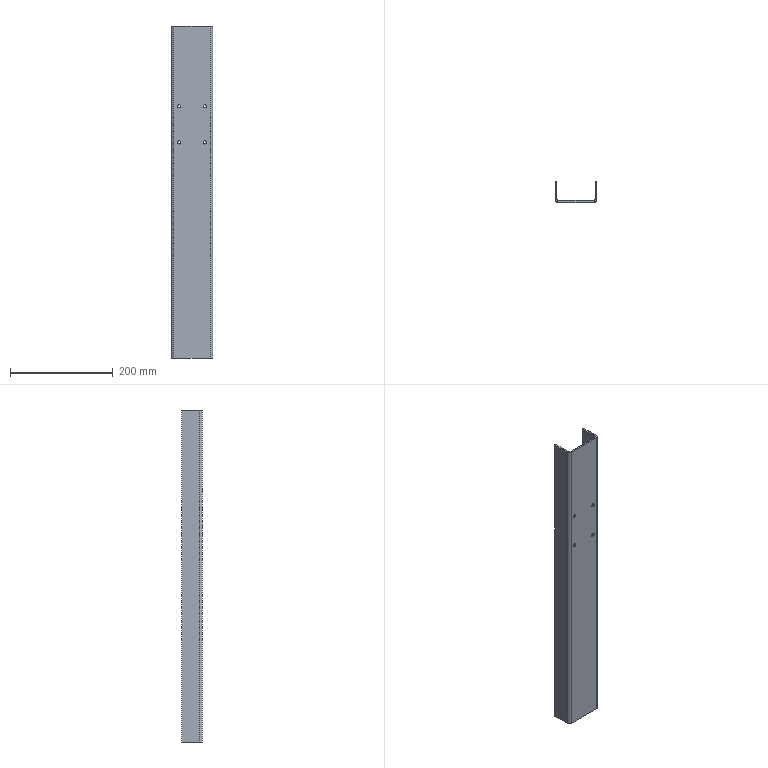Part | SolidWorks | features Extrusion 1, ICE 1 | 1 solid | 22 faces | box 80 x 40 x 645 mm | volume 291778 mm3 | cylinder 12 | plane 10 | commonest cylinder face diameters 6.5 x8 4 x2 10 x2
STEP:
#1=CARTESIAN_POINT('',(15.,-37.,415.75));
#2=VERTEX_POINT('',#1);
#3=CARTESIAN_POINT('',(15.,-37.,422.25));
#4=VERTEX_POINT('',#3);
#5=CARTESIAN_POINT('',(15.,-37.,419.));
#6=DIRECTION('',(0.,1.,0.));
#7=DIRECTION('',(-1.,0.,0.));
#8=AXIS2_PLACEMENT_3D('',#5,#6,#7);
#9=CIRCLE('',#8,3.25);
#10=EDGE_CURVE('',#2,#4,#9,.T.);
#11=ORIENTED_EDGE('',*,*,#10,.T.);
#12=CARTESIAN_POINT('',(15.,-40.,422.25));
#13=VERTEX_POINT('',#12);
#14=CARTESIAN_POINT('',(15.,-30.,422.25));
#15=DIRECTION('',(0.,-1.,0.));
#16=VECTOR('',#15,1000.);
#17=LINE('',#14,#16);
#18=EDGE_CURVE('',#4,#13,#17,.T.);
#19=ORIENTED_EDGE('',*,*,#18,.T.);
#20=CARTESIAN_POINT('',(15.,-40.,415.75));
#21=VERTEX_POINT('',#20);
#22=CARTESIAN_POINT('',(15.,-40.,419.));
#23=DIRECTION('',(0.,-1.,0.));
#24=DIRECTION('',(0.,0.,-1.));
#25=AXIS2_PLACEMENT_3D('',#22,#23,#24);
#26=CIRCLE('',#25,3.25);
#27=EDGE_CURVE('',#13,#21,#26,.T.);
#28=ORIENTED_EDGE('',*,*,#27,.T.);
#29=CARTESIAN_POINT('',(15.,-30.,415.75));
#30=DIRECTION('',(0.,-1.,0.));
#31=VECTOR('',#30,1000.);
#32=LINE('',#29,#31);
#33=EDGE_CURVE('',#2,#21,#32,.T.);
#34=ORIENTED_EDGE('',*,*,#33,.F.);
#35=EDGE_LOOP('',(#11,#19,#28,#34));
#36=FACE_OUTER_BOUND('',#35,.T.);
#37=CARTESIAN_POINT('',(15.,-30.,419.));
#38=DIRECTION('',(0.,-1.,0.));
#39=DIRECTION('',(0.,0.,-1.));
#40=AXIS2_PLACEMENT_3D('',#37,#38,#39);
#41=CYLINDRICAL_SURFACE('',#40,3.25);
#42=ADVANCED_FACE('',(#36),#41,.F.);
#43=CARTESIAN_POINT('',(65.,-37.,415.75));
#44=VERTEX_POINT('',#43);
#45=CARTESIAN_POINT('',(65.,-37.,422.25));
#46=VERTEX_POINT('',#45);
#47=CARTESIAN_POINT('',(65.,-37.,419.));
#48=DIRECTION('',(0.,1.,0.));
#49=DIRECTION('',(-1.,0.,0.));
#50=AXIS2_PLACEMENT_3D('',#47,#48,#49);
#51=CIRCLE('',#50,3.25);
#52=EDGE_CURVE('',#44,#46,#51,.T.);
#53=ORIENTED_EDGE('',*,*,#52,.T.);
#54=CARTESIAN_POINT('',(65.,-40.,422.25));
#55=VERTEX_POINT('',#54);
#56=CARTESIAN_POINT('',(65.,-30.,422.25));
#57=DIRECTION('',(0.,-1.,0.));
#58=VECTOR('',#57,1000.);
#59=LINE('',#56,#58);
#60=EDGE_CURVE('',#46,#55,#59,.T.);
#61=ORIENTED_EDGE('',*,*,#60,.T.);
#62=CARTESIAN_POINT('',(65.,-40.,415.75));
#63=VERTEX_POINT('',#62);
#64=CARTESIAN_POINT('',(65.,-40.,419.));
#65=DIRECTION('',(0.,-1.,0.));
#66=DIRECTION('',(0.,0.,-1.));
#67=AXIS2_PLACEMENT_3D('',#64,#65,#66);
#68=CIRCLE('',#67,3.25);
#69=EDGE_CURVE('',#55,#63,#68,.T.);
#70=ORIENTED_EDGE('',*,*,#69,.T.);
#71=CARTESIAN_POINT('',(65.,-30.,415.75));
#72=DIRECTION('',(0.,-1.,0.));
#73=VECTOR('',#72,1000.);
#74=LINE('',#71,#73);
#75=EDGE_CURVE('',#44,#63,#74,.T.);
#76=ORIENTED_EDGE('',*,*,#75,.F.);
#77=EDGE_LOOP('',(#53,#61,#70,#76));
#78=FACE_OUTER_BOUND('',#77,.T.);
#79=CARTESIAN_POINT('',(65.,-30.,419.));
#80=DIRECTION('',(0.,-1.,0.));
#81=DIRECTION('',(0.,0.,-1.));
#82=AXIS2_PLACEMENT_3D('',#79,#80,#81);
#83=CYLINDRICAL_SURFACE('',#82,3.25);
#84=ADVANCED_FACE('',(#78),#83,.F.);
#85=CARTESIAN_POINT('',(65.,-37.,485.75));
#86=VERTEX_POINT('',#85);
#87=CARTESIAN_POINT('',(65.,-37.,492.25));
#88=VERTEX_POINT('',#87);
#89=CARTESIAN_POINT('',(65.,-37.,489.));
#90=DIRECTION('',(0.,1.,0.));
#91=DIRECTION('',(-1.,0.,0.));
#92=AXIS2_PLACEMENT_3D('',#89,#90,#91);
#93=CIRCLE('',#92,3.25);
#94=EDGE_CURVE('',#86,#88,#93,.T.);
#95=ORIENTED_EDGE('',*,*,#94,.T.);
#96=CARTESIAN_POINT('',(65.,-40.,492.25));
#97=VERTEX_POINT('',#96);
#98=CARTESIAN_POINT('',(65.,-30.,492.25));
#99=DIRECTION('',(0.,-1.,0.));
#100=VECTOR('',#99,1000.);
#101=LINE('',#98,#100);
#102=EDGE_CURVE('',#88,#97,#101,.T.);
#103=ORIENTED_EDGE('',*,*,#102,.T.);
#104=CARTESIAN_POINT('',(65.,-40.,485.75));
#105=VERTEX_POINT('',#104);
#106=CARTESIAN_POINT('',(65.,-40.,489.));
#107=DIRECTION('',(0.,-1.,0.));
#108=DIRECTION('',(0.,0.,-1.));
#109=AXIS2_PLACEMENT_3D('',#106,#107,#108);
#110=CIRCLE('',#109,3.25);
#111=EDGE_CURVE('',#97,#105,#110,.T.);
#112=ORIENTED_EDGE('',*,*,#111,.T.);
#113=CARTESIAN_POINT('',(65.,-30.,485.75));
#114=DIRECTION('',(0.,-1.,0.));
#115=VECTOR('',#114,1000.);
#116=LINE('',#113,#115);
#117=EDGE_CURVE('',#86,#105,#116,.T.);
#118=ORIENTED_EDGE('',*,*,#117,.F.);
#119=EDGE_LOOP('',(#95,#103,#112,#118));
#120=FACE_OUTER_BOUND('',#119,.T.);
#121=CARTESIAN_POINT('',(65.,-30.,489.));
#122=DIRECTION('',(0.,-1.,0.));
#123=DIRECTION('',(0.,0.,-1.));
#124=AXIS2_PLACEMENT_3D('',#121,#122,#123);
#125=CYLINDRICAL_SURFACE('',#124,3.25);
#126=ADVANCED_FACE('',(#120),#125,.F.);
#127=CARTESIAN_POINT('',(15.,-37.,485.75));
#128=VERTEX_POINT('',#127);
#129=CARTESIAN_POINT('',(15.,-37.,492.25));
#130=VERTEX_POINT('',#129);
#131=CARTESIAN_POINT('',(15.,-37.,489.));
#132=DIRECTION('',(0.,1.,0.));
#133=DIRECTION('',(-1.,0.,0.));
#134=AXIS2_PLACEMENT_3D('',#131,#132,#133);
#135=CIRCLE('',#134,3.25);
#136=EDGE_CURVE('',#128,#130,#135,.T.);
#137=ORIENTED_EDGE('',*,*,#136,.T.);
#138=CARTESIAN_POINT('',(15.,-40.,492.25));
#139=VERTEX_POINT('',#138);
#140=CARTESIAN_POINT('',(15.,-30.,492.25));
#141=DIRECTION('',(0.,-1.,0.));
#142=VECTOR('',#141,1000.);
#143=LINE('',#140,#142);
#144=EDGE_CURVE('',#130,#139,#143,.T.);
#145=ORIENTED_EDGE('',*,*,#144,.T.);
#146=CARTESIAN_POINT('',(15.,-40.,485.75));
#147=VERTEX_POINT('',#146);
#148=CARTESIAN_POINT('',(15.,-40.,489.));
#149=DIRECTION('',(0.,-1.,0.));
#150=DIRECTION('',(0.,0.,-1.));
#151=AXIS2_PLACEMENT_3D('',#148,#149,#150);
#152=CIRCLE('',#151,3.25);
#153=EDGE_CURVE('',#139,#147,#152,.T.);
#154=ORIENTED_EDGE('',*,*,#153,.T.);
#155=CARTESIAN_POINT('',(15.,-30.,485.75));
#156=DIRECTION('',(0.,-1.,0.));
#157=VECTOR('',#156,1000.);
#158=LINE('',#155,#157);
#159=EDGE_CURVE('',#128,#147,#158,.T.);
#160=ORIENTED_EDGE('',*,*,#159,.F.);
#161=EDGE_LOOP('',(#137,#145,#154,#160));
#162=FACE_OUTER_BOUND('',#161,.T.);
#163=CARTESIAN_POINT('',(15.,-30.,489.));
#164=DIRECTION('',(0.,-1.,0.));
#165=DIRECTION('',(0.,0.,-1.));
#166=AXIS2_PLACEMENT_3D('',#163,#164,#165);
#167=CYLINDRICAL_SURFACE('',#166,3.25);
#168=ADVANCED_FACE('',(#162),#167,.F.);
#169=CARTESIAN_POINT('',(80.,-35.,0.));
#170=VERTEX_POINT('',#169);
#171=CARTESIAN_POINT('',(80.,0.,0.));
#172=VERTEX_POINT('',#171);
#173=CARTESIAN_POINT('',(80.,-35.,0.));
#174=DIRECTION('',(0.,1.,0.));
#175=VECTOR('',#174,1000.);
#176=LINE('',#173,#175);
#177=EDGE_CURVE('',#170,#172,#176,.T.);
#178=ORIENTED_EDGE('',*,*,#177,.T.);
#179=CARTESIAN_POINT('',(80.,0.,645.));
#180=VERTEX_POINT('',#179);
#181=CARTESIAN_POINT('',(80.,0.,645.));
#182=DIRECTION('',(0.,0.,-1.));
#183=VECTOR('',#182,1000.);
#184=LINE('',#181,#183);
#185=EDGE_CURVE('',#180,#172,#184,.T.);
#186=ORIENTED_EDGE('',*,*,#185,.F.);
#187=CARTESIAN_POINT('',(80.,-35.,645.));
#188=VERTEX_POINT('',#187);
#189=CARTESIAN_POINT('',(80.,-35.,645.));
#190=DIRECTION('',(0.,1.,0.));
#191=VECTOR('',#190,1000.);
#192=LINE('',#189,#191);
#193=EDGE_CURVE('',#188,#180,#192,.T.);
#194=ORIENTED_EDGE('',*,*,#193,.F.);
#195=CARTESIAN_POINT('',(80.,-35.,645.));
#196=DIRECTION('',(0.,0.,-1.));
#197=VECTOR('',#196,1000.);
#198=LINE('',#195,#197);
#199=EDGE_CURVE('',#188,#170,#198,.T.);
#200=ORIENTED_EDGE('',*,*,#199,.T.);
#201=EDGE_LOOP('',(#178,#186,#194,#200));
#202=FACE_OUTER_BOUND('',#201,.T.);
#203=CARTESIAN_POINT('',(80.,-35.,645.));
#204=DIRECTION('',(-1.,0.,0.));
#205=DIRECTION('',(0.,0.,1.));
#206=AXIS2_PLACEMENT_3D('',#203,#204,#205);
#207=PLANE('',#206);
#208=ADVANCED_FACE('',(#202),#207,.F.);
#209=CARTESIAN_POINT('',(77.,0.,0.));
#210=VERTEX_POINT('',#209);
#211=CARTESIAN_POINT('',(80.,0.,0.));
#212=DIRECTION('',(-1.,0.,0.));
#213=VECTOR('',#212,1000.);
#214=LINE('',#211,#213);
#215=EDGE_CURVE('',#172,#210,#214,.T.);
#216=ORIENTED_EDGE('',*,*,#215,.T.);
#217=CARTESIAN_POINT('',(77.,0.,645.));
#218=VERTEX_POINT('',#217);
#219=CARTESIAN_POINT('',(77.,0.,645.));
#220=DIRECTION('',(0.,0.,-1.));
#221=VECTOR('',#220,1000.);
#222=LINE('',#219,#221);
#223=EDGE_CURVE('',#218,#210,#222,.T.);
#224=ORIENTED_EDGE('',*,*,#223,.F.);
#225=CARTESIAN_POINT('',(80.,0.,645.));
#226=DIRECTION('',(-1.,0.,0.));
#227=VECTOR('',#226,1000.);
#228=LINE('',#225,#227);
#229=EDGE_CURVE('',#180,#218,#228,.T.);
#230=ORIENTED_EDGE('',*,*,#229,.F.);
#231=ORIENTED_EDGE('',*,*,#185,.T.);
#232=EDGE_LOOP('',(#216,#224,#230,#231));
#233=FACE_OUTER_BOUND('',#232,.T.);
#234=CARTESIAN_POINT('',(80.,0.,645.));
#235=DIRECTION('',(0.,-1.,0.));
#236=DIRECTION('',(0.,0.,-1.));
#237=AXIS2_PLACEMENT_3D('',#234,#235,#236);
#238=PLANE('',#237);
#239=ADVANCED_FACE('',(#233),#238,.F.);
#240=CARTESIAN_POINT('',(77.,-35.,0.));
#241=VERTEX_POINT('',#240);
#242=CARTESIAN_POINT('',(77.,-35.,0.));
#243=DIRECTION('',(0.,1.,0.));
#244=VECTOR('',#243,1000.);
#245=LINE('',#242,#244);
#246=EDGE_CURVE('',#241,#210,#245,.T.);
#247=ORIENTED_EDGE('',*,*,#246,.F.);
#248=CARTESIAN_POINT('',(77.,-35.,645.));
#249=VERTEX_POINT('',#248);
#250=CARTESIAN_POINT('',(77.,-35.,645.));
#251=DIRECTION('',(0.,0.,-1.));
#252=VECTOR('',#251,1000.);
#253=LINE('',#250,#252);
#254=EDGE_CURVE('',#249,#241,#253,.T.);
#255=ORIENTED_EDGE('',*,*,#254,.F.);
#256=CARTESIAN_POINT('',(77.,-35.,645.));
#257=DIRECTION('',(0.,1.,0.));
#258=VECTOR('',#257,1000.);
#259=LINE('',#256,#258);
#260=EDGE_CURVE('',#249,#218,#259,.T.);
#261=ORIENTED_EDGE('',*,*,#260,.T.);
#262=ORIENTED_EDGE('',*,*,#223,.T.);
#263=EDGE_LOOP('',(#247,#255,#261,#262));
#264=FACE_OUTER_BOUND('',#263,.T.);
#265=CARTESIAN_POINT('',(77.,-35.,645.));
#266=DIRECTION('',(-1.,0.,0.));
#267=DIRECTION('',(0.,0.,1.));
#268=AXIS2_PLACEMENT_3D('',#265,#266,#267);
#269=PLANE('',#268);
#270=ADVANCED_FACE('',(#264),#269,.T.);
#271=CARTESIAN_POINT('',(75.,-37.,0.));
#272=VERTEX_POINT('',#271);
#273=CARTESIAN_POINT('',(75.,-35.,0.));
#274=DIRECTION('',(0.,0.,1.));
#275=DIRECTION('',(1.,0.,0.));
#276=AXIS2_PLACEMENT_3D('',#273,#274,#275);
#277=CIRCLE('',#276,2.);
#278=EDGE_CURVE('',#272,#241,#277,.T.);
#279=ORIENTED_EDGE('',*,*,#278,.F.);
#280=CARTESIAN_POINT('',(75.,-37.,645.));
#281=VERTEX_POINT('',#280);
#282=CARTESIAN_POINT('',(75.,-37.,645.));
#283=DIRECTION('',(0.,0.,-1.));
#284=VECTOR('',#283,1000.);
#285=LINE('',#282,#284);
#286=EDGE_CURVE('',#281,#272,#285,.T.);
#287=ORIENTED_EDGE('',*,*,#286,.F.);
#288=CARTESIAN_POINT('',(75.,-35.,645.));
#289=DIRECTION('',(0.,0.,1.));
#290=DIRECTION('',(1.,0.,0.));
#291=AXIS2_PLACEMENT_3D('',#288,#289,#290);
#292=CIRCLE('',#291,2.);
#293=EDGE_CURVE('',#281,#249,#292,.T.);
#294=ORIENTED_EDGE('',*,*,#293,.T.);
#295=ORIENTED_EDGE('',*,*,#254,.T.);
#296=EDGE_LOOP('',(#279,#287,#294,#295));
#297=FACE_OUTER_BOUND('',#296,.T.);
#298=CARTESIAN_POINT('',(75.,-35.,645.));
#299=DIRECTION('',(0.,0.,-1.));
#300=DIRECTION('',(-1.,0.,0.));
#301=AXIS2_PLACEMENT_3D('',#298,#299,#300);
#302=CYLINDRICAL_SURFACE('',#301,2.);
#303=ADVANCED_FACE('',(#297),#302,.F.);
#304=ORIENTED_EDGE('',*,*,#10,.F.);
#305=CARTESIAN_POINT('',(15.,-37.,419.));
#306=DIRECTION('',(0.,1.,0.));
#307=DIRECTION('',(-1.,0.,0.));
#308=AXIS2_PLACEMENT_3D('',#305,#306,#307);
#309=CIRCLE('',#308,3.25);
#310=EDGE_CURVE('',#4,#2,#309,.T.);
#311=ORIENTED_EDGE('',*,*,#310,.F.);
#312=EDGE_LOOP('',(#304,#311));
#313=FACE_BOUND('',#312,.T.);
#314=ORIENTED_EDGE('',*,*,#52,.F.);
#315=CARTESIAN_POINT('',(65.,-37.,419.));
#316=DIRECTION('',(0.,1.,0.));
#317=DIRECTION('',(-1.,0.,0.));
#318=AXIS2_PLACEMENT_3D('',#315,#316,#317);
#319=CIRCLE('',#318,3.25);
#320=EDGE_CURVE('',#46,#44,#319,.T.);
#321=ORIENTED_EDGE('',*,*,#320,.F.);
#322=EDGE_LOOP('',(#314,#321));
#323=FACE_BOUND('',#322,.T.);
#324=ORIENTED_EDGE('',*,*,#94,.F.);
#325=CARTESIAN_POINT('',(65.,-37.,489.));
#326=DIRECTION('',(0.,1.,0.));
#327=DIRECTION('',(-1.,0.,0.));
#328=AXIS2_PLACEMENT_3D('',#325,#326,#327);
#329=CIRCLE('',#328,3.25);
#330=EDGE_CURVE('',#88,#86,#329,.T.);
#331=ORIENTED_EDGE('',*,*,#330,.F.);
#332=EDGE_LOOP('',(#324,#331));
#333=FACE_BOUND('',#332,.T.);
#334=ORIENTED_EDGE('',*,*,#136,.F.);
#335=CARTESIAN_POINT('',(15.,-37.,489.));
#336=DIRECTION('',(0.,1.,0.));
#337=DIRECTION('',(-1.,0.,0.));
#338=AXIS2_PLACEMENT_3D('',#335,#336,#337);
#339=CIRCLE('',#338,3.25);
#340=EDGE_CURVE('',#130,#128,#339,.T.);
#341=ORIENTED_EDGE('',*,*,#340,.F.);
#342=EDGE_LOOP('',(#334,#341));
#343=FACE_BOUND('',#342,.T.);
#344=CARTESIAN_POINT('',(5.,-37.,0.));
#345=VERTEX_POINT('',#344);
#346=CARTESIAN_POINT('',(5.,-37.,0.));
#347=DIRECTION('',(1.,0.,0.));
#348=VECTOR('',#347,1000.);
#349=LINE('',#346,#348);
#350=EDGE_CURVE('',#345,#272,#349,.T.);
#351=ORIENTED_EDGE('',*,*,#350,.F.);
#352=CARTESIAN_POINT('',(5.,-37.,645.));
#353=VERTEX_POINT('',#352);
#354=CARTESIAN_POINT('',(5.,-37.,645.));
#355=DIRECTION('',(0.,0.,-1.));
#356=VECTOR('',#355,1000.);
#357=LINE('',#354,#356);
#358=EDGE_CURVE('',#353,#345,#357,.T.);
#359=ORIENTED_EDGE('',*,*,#358,.F.);
#360=CARTESIAN_POINT('',(5.,-37.,645.));
#361=DIRECTION('',(1.,0.,0.));
#362=VECTOR('',#361,1000.);
#363=LINE('',#360,#362);
#364=EDGE_CURVE('',#353,#281,#363,.T.);
#365=ORIENTED_EDGE('',*,*,#364,.T.);
#366=ORIENTED_EDGE('',*,*,#286,.T.);
#367=EDGE_LOOP('',(#351,#359,#365,#366));
#368=FACE_OUTER_BOUND('',#367,.T.);
#369=CARTESIAN_POINT('',(5.,-37.,645.));
#370=DIRECTION('',(0.,1.,0.));
#371=DIRECTION('',(-1.,0.,0.));
#372=AXIS2_PLACEMENT_3D('',#369,#370,#371);
#373=PLANE('',#372);
#374=ADVANCED_FACE('',(#313,#323,#333,#343,#368),#373,.T.);
#375=CARTESIAN_POINT('',(3.,-35.,0.));
#376=VERTEX_POINT('',#375);
#377=CARTESIAN_POINT('',(5.,-35.,0.));
#378=DIRECTION('',(0.,0.,1.));
#379=DIRECTION('',(1.,0.,0.));
#380=AXIS2_PLACEMENT_3D('',#377,#378,#379);
#381=CIRCLE('',#380,2.);
#382=EDGE_CURVE('',#376,#345,#381,.T.);
#383=ORIENTED_EDGE('',*,*,#382,.F.);
#384=CARTESIAN_POINT('',(3.,-35.,645.));
#385=VERTEX_POINT('',#384);
#386=CARTESIAN_POINT('',(3.,-35.,645.));
#387=DIRECTION('',(0.,0.,-1.));
#388=VECTOR('',#387,1000.);
#389=LINE('',#386,#388);
#390=EDGE_CURVE('',#385,#376,#389,.T.);
#391=ORIENTED_EDGE('',*,*,#390,.F.);
#392=CARTESIAN_POINT('',(5.,-35.,645.));
#393=DIRECTION('',(0.,0.,1.));
#394=DIRECTION('',(1.,0.,0.));
#395=AXIS2_PLACEMENT_3D('',#392,#393,#394);
#396=CIRCLE('',#395,2.);
#397=EDGE_CURVE('',#385,#353,#396,.T.);
#398=ORIENTED_EDGE('',*,*,#397,.T.);
#399=ORIENTED_EDGE('',*,*,#358,.T.);
#400=EDGE_LOOP('',(#383,#391,#398,#399));
#401=FACE_OUTER_BOUND('',#400,.T.);
#402=CARTESIAN_POINT('',(5.,-35.,645.));
#403=DIRECTION('',(0.,0.,-1.));
#404=DIRECTION('',(-1.,0.,0.));
#405=AXIS2_PLACEMENT_3D('',#402,#403,#404);
#406=CYLINDRICAL_SURFACE('',#405,2.);
#407=ADVANCED_FACE('',(#401),#406,.F.);
#408=CARTESIAN_POINT('',(3.,0.,0.));
#409=VERTEX_POINT('',#408);
#410=CARTESIAN_POINT('',(3.,0.,0.));
#411=DIRECTION('',(0.,-1.,0.));
#412=VECTOR('',#411,1000.);
#413=LINE('',#410,#412);
#414=EDGE_CURVE('',#409,#376,#413,.T.);
#415=ORIENTED_EDGE('',*,*,#414,.F.);
#416=CARTESIAN_POINT('',(3.,0.,645.));
#417=VERTEX_POINT('',#416);
#418=CARTESIAN_POINT('',(3.,0.,645.));
#419=DIRECTION('',(0.,0.,-1.));
#420=VECTOR('',#419,1000.);
#421=LINE('',#418,#420);
#422=EDGE_CURVE('',#417,#409,#421,.T.);
#423=ORIENTED_EDGE('',*,*,#422,.F.);
#424=CARTESIAN_POINT('',(3.,0.,645.));
#425=DIRECTION('',(0.,-1.,0.));
#426=VECTOR('',#425,1000.);
#427=LINE('',#424,#426);
#428=EDGE_CURVE('',#417,#385,#427,.T.);
#429=ORIENTED_EDGE('',*,*,#428,.T.);
#430=ORIENTED_EDGE('',*,*,#390,.T.);
#431=EDGE_LOOP('',(#415,#423,#429,#430));
#432=FACE_OUTER_BOUND('',#431,.T.);
#433=CARTESIAN_POINT('',(3.,0.,645.));
#434=DIRECTION('',(1.,0.,0.));
#435=DIRECTION('',(0.,0.,-1.));
#436=AXIS2_PLACEMENT_3D('',#433,#434,#435);
#437=PLANE('',#436);
#438=ADVANCED_FACE('',(#432),#437,.T.);
#439=CARTESIAN_POINT('',(0.,0.,0.));
#440=VERTEX_POINT('',#439);
#441=CARTESIAN_POINT('',(3.,0.,0.));
#442=DIRECTION('',(-1.,0.,0.));
#443=VECTOR('',#442,1000.);
#444=LINE('',#441,#443);
#445=EDGE_CURVE('',#409,#440,#444,.T.);
#446=ORIENTED_EDGE('',*,*,#445,.T.);
#447=CARTESIAN_POINT('',(0.,0.,645.));
#448=VERTEX_POINT('',#447);
#449=CARTESIAN_POINT('',(0.,0.,645.));
#450=DIRECTION('',(0.,0.,-1.));
#451=VECTOR('',#450,1000.);
#452=LINE('',#449,#451);
#453=EDGE_CURVE('',#448,#440,#452,.T.);
#454=ORIENTED_EDGE('',*,*,#453,.F.);
#455=CARTESIAN_POINT('',(3.,0.,645.));
#456=DIRECTION('',(-1.,0.,0.));
#457=VECTOR('',#456,1000.);
#458=LINE('',#455,#457);
#459=EDGE_CURVE('',#417,#448,#458,.T.);
#460=ORIENTED_EDGE('',*,*,#459,.F.);
#461=ORIENTED_EDGE('',*,*,#422,.T.);
#462=EDGE_LOOP('',(#446,#454,#460,#461));
#463=FACE_OUTER_BOUND('',#462,.T.);
#464=CARTESIAN_POINT('',(3.,0.,645.));
#465=DIRECTION('',(0.,-1.,0.));
#466=DIRECTION('',(0.,0.,-1.));
#467=AXIS2_PLACEMENT_3D('',#464,#465,#466);
#468=PLANE('',#467);
#469=ADVANCED_FACE('',(#463),#468,.F.);
#470=CARTESIAN_POINT('',(0.,-35.,0.));
#471=VERTEX_POINT('',#470);
#472=CARTESIAN_POINT('',(0.,0.,0.));
#473=DIRECTION('',(0.,-1.,0.));
#474=VECTOR('',#473,1000.);
#475=LINE('',#472,#474);
#476=EDGE_CURVE('',#440,#471,#475,.T.);
#477=ORIENTED_EDGE('',*,*,#476,.T.);
#478=CARTESIAN_POINT('',(0.,-35.,645.));
#479=VERTEX_POINT('',#478);
#480=CARTESIAN_POINT('',(0.,-35.,645.));
#481=DIRECTION('',(0.,0.,-1.));
#482=VECTOR('',#481,1000.);
#483=LINE('',#480,#482);
#484=EDGE_CURVE('',#479,#471,#483,.T.);
#485=ORIENTED_EDGE('',*,*,#484,.F.);
#486=CARTESIAN_POINT('',(0.,0.,645.));
#487=DIRECTION('',(0.,-1.,0.));
#488=VECTOR('',#487,1000.);
#489=LINE('',#486,#488);
#490=EDGE_CURVE('',#448,#479,#489,.T.);
#491=ORIENTED_EDGE('',*,*,#490,.F.);
#492=ORIENTED_EDGE('',*,*,#453,.T.);
#493=EDGE_LOOP('',(#477,#485,#491,#492));
#494=FACE_OUTER_BOUND('',#493,.T.);
#495=CARTESIAN_POINT('',(0.,0.,645.));
#496=DIRECTION('',(1.,0.,0.));
#497=DIRECTION('',(0.,1.,0.));
#498=AXIS2_PLACEMENT_3D('',#495,#496,#497);
#499=PLANE('',#498);
#500=ADVANCED_FACE('',(#494),#499,.F.);
#501=CARTESIAN_POINT('',(5.,-40.,0.));
#502=VERTEX_POINT('',#501);
#503=CARTESIAN_POINT('',(5.,-35.,0.));
#504=DIRECTION('',(0.,0.,1.));
#505=DIRECTION('',(1.,0.,0.));
#506=AXIS2_PLACEMENT_3D('',#503,#504,#505);
#507=CIRCLE('',#506,5.);
#508=EDGE_CURVE('',#471,#502,#507,.T.);
#509=ORIENTED_EDGE('',*,*,#508,.T.);
#510=CARTESIAN_POINT('',(5.,-40.,645.));
#511=VERTEX_POINT('',#510);
#512=CARTESIAN_POINT('',(5.,-40.,645.));
#513=DIRECTION('',(0.,0.,-1.));
#514=VECTOR('',#513,1000.);
#515=LINE('',#512,#514);
#516=EDGE_CURVE('',#511,#502,#515,.T.);
#517=ORIENTED_EDGE('',*,*,#516,.F.);
#518=CARTESIAN_POINT('',(5.,-35.,645.));
#519=DIRECTION('',(0.,0.,1.));
#520=DIRECTION('',(1.,0.,0.));
#521=AXIS2_PLACEMENT_3D('',#518,#519,#520);
#522=CIRCLE('',#521,5.);
#523=EDGE_CURVE('',#479,#511,#522,.T.);
#524=ORIENTED_EDGE('',*,*,#523,.F.);
#525=ORIENTED_EDGE('',*,*,#484,.T.);
#526=EDGE_LOOP('',(#509,#517,#524,#525));
#527=FACE_OUTER_BOUND('',#526,.T.);
#528=CARTESIAN_POINT('',(5.,-35.,645.));
#529=DIRECTION('',(0.,0.,-1.));
#530=DIRECTION('',(-1.,0.,0.));
#531=AXIS2_PLACEMENT_3D('',#528,#529,#530);
#532=CYLINDRICAL_SURFACE('',#531,5.);
#533=ADVANCED_FACE('',(#527),#532,.T.);
#534=CARTESIAN_POINT('',(15.,-40.,419.));
#535=DIRECTION('',(0.,-1.,0.));
#536=DIRECTION('',(0.,0.,-1.));
#537=AXIS2_PLACEMENT_3D('',#534,#535,#536);
#538=CIRCLE('',#537,3.25);
#539=EDGE_CURVE('',#21,#13,#538,.T.);
#540=ORIENTED_EDGE('',*,*,#539,.F.);
#541=ORIENTED_EDGE('',*,*,#27,.F.);
#542=EDGE_LOOP('',(#540,#541));
#543=FACE_BOUND('',#542,.T.);
#544=CARTESIAN_POINT('',(65.,-40.,419.));
#545=DIRECTION('',(0.,-1.,0.));
#546=DIRECTION('',(0.,0.,-1.));
#547=AXIS2_PLACEMENT_3D('',#544,#545,#546);
#548=CIRCLE('',#547,3.25);
#549=EDGE_CURVE('',#63,#55,#548,.T.);
#550=ORIENTED_EDGE('',*,*,#549,.F.);
#551=ORIENTED_EDGE('',*,*,#69,.F.);
#552=EDGE_LOOP('',(#550,#551));
#553=FACE_BOUND('',#552,.T.);
#554=CARTESIAN_POINT('',(65.,-40.,489.));
#555=DIRECTION('',(0.,-1.,0.));
#556=DIRECTION('',(0.,0.,-1.));
#557=AXIS2_PLACEMENT_3D('',#554,#555,#556);
#558=CIRCLE('',#557,3.25);
#559=EDGE_CURVE('',#105,#97,#558,.T.);
#560=ORIENTED_EDGE('',*,*,#559,.F.);
#561=ORIENTED_EDGE('',*,*,#111,.F.);
#562=EDGE_LOOP('',(#560,#561));
#563=FACE_BOUND('',#562,.T.);
#564=CARTESIAN_POINT('',(15.,-40.,489.));
#565=DIRECTION('',(0.,-1.,0.));
#566=DIRECTION('',(0.,0.,-1.));
#567=AXIS2_PLACEMENT_3D('',#564,#565,#566);
#568=CIRCLE('',#567,3.25);
#569=EDGE_CURVE('',#147,#139,#568,.T.);
#570=ORIENTED_EDGE('',*,*,#569,.F.);
#571=ORIENTED_EDGE('',*,*,#153,.F.);
#572=EDGE_LOOP('',(#570,#571));
#573=FACE_BOUND('',#572,.T.);
#574=CARTESIAN_POINT('',(75.,-40.,0.));
#575=VERTEX_POINT('',#574);
#576=CARTESIAN_POINT('',(5.,-40.,0.));
#577=DIRECTION('',(1.,0.,0.));
#578=VECTOR('',#577,1000.);
#579=LINE('',#576,#578);
#580=EDGE_CURVE('',#502,#575,#579,.T.);
#581=ORIENTED_EDGE('',*,*,#580,.T.);
#582=CARTESIAN_POINT('',(75.,-40.,645.));
#583=VERTEX_POINT('',#582);
#584=CARTESIAN_POINT('',(75.,-40.,645.));
#585=DIRECTION('',(0.,0.,-1.));
#586=VECTOR('',#585,1000.);
#587=LINE('',#584,#586);
#588=EDGE_CURVE('',#583,#575,#587,.T.);
#589=ORIENTED_EDGE('',*,*,#588,.F.);
#590=CARTESIAN_POINT('',(5.,-40.,645.));
#591=DIRECTION('',(1.,0.,0.));
#592=VECTOR('',#591,1000.);
#593=LINE('',#590,#592);
#594=EDGE_CURVE('',#511,#583,#593,.T.);
#595=ORIENTED_EDGE('',*,*,#594,.F.);
#596=ORIENTED_EDGE('',*,*,#516,.T.);
#597=EDGE_LOOP('',(#581,#589,#595,#596));
#598=FACE_OUTER_BOUND('',#597,.T.);
#599=CARTESIAN_POINT('',(5.,-40.,645.));
#600=DIRECTION('',(0.,1.,0.));
#601=DIRECTION('',(0.,0.,1.));
#602=AXIS2_PLACEMENT_3D('',#599,#600,#601);
#603=PLANE('',#602);
#604=ADVANCED_FACE('',(#543,#553,#563,#573,#598),#603,.F.);
#605=CARTESIAN_POINT('',(75.,-35.,0.));
#606=DIRECTION('',(0.,0.,1.));
#607=DIRECTION('',(1.,0.,0.));
#608=AXIS2_PLACEMENT_3D('',#605,#606,#607);
#609=CIRCLE('',#608,5.);
#610=EDGE_CURVE('',#575,#170,#609,.T.);
#611=ORIENTED_EDGE('',*,*,#610,.T.);
#612=ORIENTED_EDGE('',*,*,#199,.F.);
#613=CARTESIAN_POINT('',(75.,-35.,645.));
#614=DIRECTION('',(0.,0.,1.));
#615=DIRECTION('',(1.,0.,0.));
#616=AXIS2_PLACEMENT_3D('',#613,#614,#615);
#617=CIRCLE('',#616,5.);
#618=EDGE_CURVE('',#583,#188,#617,.T.);
#619=ORIENTED_EDGE('',*,*,#618,.F.);
#620=ORIENTED_EDGE('',*,*,#588,.T.);
#621=EDGE_LOOP('',(#611,#612,#619,#620));
#622=FACE_OUTER_BOUND('',#621,.T.);
#623=CARTESIAN_POINT('',(75.,-35.,645.));
#624=DIRECTION('',(0.,0.,-1.));
#625=DIRECTION('',(-1.,0.,0.));
#626=AXIS2_PLACEMENT_3D('',#623,#624,#625);
#627=CYLINDRICAL_SURFACE('',#626,5.);
#628=ADVANCED_FACE('',(#622),#627,.T.);
#629=ORIENTED_EDGE('',*,*,#193,.T.);
#630=ORIENTED_EDGE('',*,*,#229,.T.);
#631=ORIENTED_EDGE('',*,*,#260,.F.);
#632=ORIENTED_EDGE('',*,*,#293,.F.);
#633=ORIENTED_EDGE('',*,*,#364,.F.);
#634=ORIENTED_EDGE('',*,*,#397,.F.);
#635=ORIENTED_EDGE('',*,*,#428,.F.);
#636=ORIENTED_EDGE('',*,*,#459,.T.);
#637=ORIENTED_EDGE('',*,*,#490,.T.);
#638=ORIENTED_EDGE('',*,*,#523,.T.);
#639=ORIENTED_EDGE('',*,*,#594,.T.);
#640=ORIENTED_EDGE('',*,*,#618,.T.);
#641=EDGE_LOOP('',(#629,#630,#631,#632,#633,#634,#635,#636,#637,#638,#639,#640));
#642=FACE_OUTER_BOUND('',#641,.T.);
#643=CARTESIAN_POINT('',(75.,-35.,645.));
#644=DIRECTION('',(0.,0.,1.));
#645=DIRECTION('',(1.,0.,0.));
#646=AXIS2_PLACEMENT_3D('',#643,#644,#645);
#647=PLANE('',#646);
#648=ADVANCED_FACE('',(#642),#647,.T.);
#649=ORIENTED_EDGE('',*,*,#177,.F.);
#650=ORIENTED_EDGE('',*,*,#610,.F.);
#651=ORIENTED_EDGE('',*,*,#580,.F.);
#652=ORIENTED_EDGE('',*,*,#508,.F.);
#653=ORIENTED_EDGE('',*,*,#476,.F.);
#654=ORIENTED_EDGE('',*,*,#445,.F.);
#655=ORIENTED_EDGE('',*,*,#414,.T.);
#656=ORIENTED_EDGE('',*,*,#382,.T.);
#657=ORIENTED_EDGE('',*,*,#350,.T.);
#658=ORIENTED_EDGE('',*,*,#278,.T.);
#659=ORIENTED_EDGE('',*,*,#246,.T.);
#660=ORIENTED_EDGE('',*,*,#215,.F.);
#661=EDGE_LOOP('',(#649,#650,#651,#652,#653,#654,#655,#656,#657,#658,#659,#660));
#662=FACE_OUTER_BOUND('',#661,.T.);
#663=CARTESIAN_POINT('',(75.,-35.,0.));
#664=DIRECTION('',(0.,0.,1.));
#665=DIRECTION('',(1.,0.,0.));
#666=AXIS2_PLACEMENT_3D('',#663,#664,#665);
#667=PLANE('',#666);
#668=ADVANCED_FACE('',(#662),#667,.F.);
#669=ORIENTED_EDGE('',*,*,#144,.F.);
#670=ORIENTED_EDGE('',*,*,#340,.T.);
#671=ORIENTED_EDGE('',*,*,#159,.T.);
#672=ORIENTED_EDGE('',*,*,#569,.T.);
#673=EDGE_LOOP('',(#669,#670,#671,#672));
#674=FACE_OUTER_BOUND('',#673,.T.);
#675=CARTESIAN_POINT('',(15.,-30.,489.));
#676=DIRECTION('',(0.,-1.,0.));
#677=DIRECTION('',(0.,0.,-1.));
#678=AXIS2_PLACEMENT_3D('',#675,#676,#677);
#679=CYLINDRICAL_SURFACE('',#678,3.25);
#680=ADVANCED_FACE('',(#674),#679,.F.);
#681=ORIENTED_EDGE('',*,*,#102,.F.);
#682=ORIENTED_EDGE('',*,*,#330,.T.);
#683=ORIENTED_EDGE('',*,*,#117,.T.);
#684=ORIENTED_EDGE('',*,*,#559,.T.);
#685=EDGE_LOOP('',(#681,#682,#683,#684));
#686=FACE_OUTER_BOUND('',#685,.T.);
#687=CARTESIAN_POINT('',(65.,-30.,489.));
#688=DIRECTION('',(0.,-1.,0.));
#689=DIRECTION('',(0.,0.,-1.));
#690=AXIS2_PLACEMENT_3D('',#687,#688,#689);
#691=CYLINDRICAL_SURFACE('',#690,3.25);
#692=ADVANCED_FACE('',(#686),#691,.F.);
#693=ORIENTED_EDGE('',*,*,#60,.F.);
#694=ORIENTED_EDGE('',*,*,#320,.T.);
#695=ORIENTED_EDGE('',*,*,#75,.T.);
#696=ORIENTED_EDGE('',*,*,#549,.T.);
#697=EDGE_LOOP('',(#693,#694,#695,#696));
#698=FACE_OUTER_BOUND('',#697,.T.);
#699=CARTESIAN_POINT('',(65.,-30.,419.));
#700=DIRECTION('',(0.,-1.,0.));
#701=DIRECTION('',(0.,0.,-1.));
#702=AXIS2_PLACEMENT_3D('',#699,#700,#701);
#703=CYLINDRICAL_SURFACE('',#702,3.25);
#704=ADVANCED_FACE('',(#698),#703,.F.);
#705=ORIENTED_EDGE('',*,*,#18,.F.);
#706=ORIENTED_EDGE('',*,*,#310,.T.);
#707=ORIENTED_EDGE('',*,*,#33,.T.);
#708=ORIENTED_EDGE('',*,*,#539,.T.);
#709=EDGE_LOOP('',(#705,#706,#707,#708));
#710=FACE_OUTER_BOUND('',#709,.T.);
#711=CARTESIAN_POINT('',(15.,-30.,419.));
#712=DIRECTION('',(0.,-1.,0.));
#713=DIRECTION('',(0.,0.,-1.));
#714=AXIS2_PLACEMENT_3D('',#711,#712,#713);
#715=CYLINDRICAL_SURFACE('',#714,3.25);
#716=ADVANCED_FACE('',(#710),#715,.F.);
#717=CLOSED_SHELL('',(#42,#84,#126,#168,#208,#239,#270,#303,#374,#407,#438,#469,#500,#533,#604,#628,#648,#668,#680,#692,#704,#716));
#718=MANIFOLD_SOLID_BREP('',#717);
#719=CARTESIAN_POINT('',(0.,0.,0.));
#720=DIRECTION('',(0.,0.,1.));
#721=DIRECTION('',(1.,0.,0.));
#722=AXIS2_PLACEMENT_3D('',#719,#720,#721);
#723=(LENGTH_UNIT()NAMED_UNIT(*)SI_UNIT(.MILLI.,.METRE.));
#724=UNCERTAINTY_MEASURE_WITH_UNIT(LENGTH_MEASURE(0.00001),#723,'','');
#725=(NAMED_UNIT(*)PLANE_ANGLE_UNIT()SI_UNIT($,.RADIAN.));
#726=(NAMED_UNIT(*)SI_UNIT($,.STERADIAN.)SOLID_ANGLE_UNIT());
#727=(GEOMETRIC_REPRESENTATION_CONTEXT(3)GLOBAL_UNCERTAINTY_ASSIGNED_CONTEXT((#724))GLOBAL_UNIT_ASSIGNED_CONTEXT((#723,#725,#726))REPRESENTATION_CONTEXT('',''));
#728=ADVANCED_BREP_SHAPE_REPRESENTATION('',(#718,#722),#727);